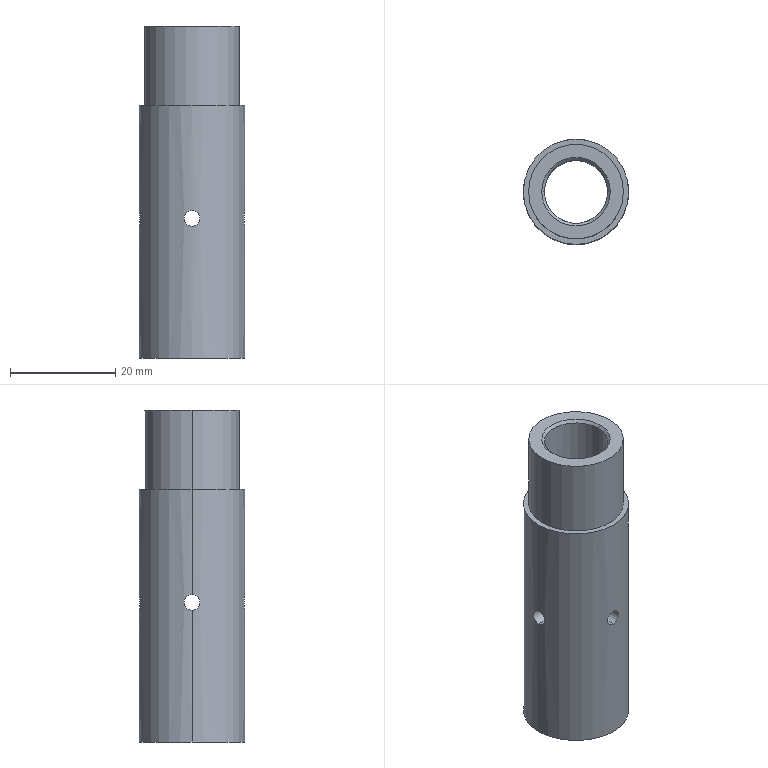Part | SolidWorks | features ICE 2, Chamfer 1, CirPattern 1, Extrusion 1, RevCut 1 | 1 solid | 19 faces | box 20 x 20 x 63 mm | volume 11653 mm3 | cylinder 14 | plane 3 | cone 2 | commonest cylinder face diameters 3 x8 12 x2 18 x2 20 x2
STEP:
#1=CARTESIAN_POINT('',(-6.,0.,62.5));
#2=VERTEX_POINT('',#1);
#3=CARTESIAN_POINT('',(6.,0.,62.5));
#4=VERTEX_POINT('',#3);
#5=CARTESIAN_POINT('',(0.,0.,62.5));
#6=DIRECTION('',(0.,0.,1.));
#7=DIRECTION('',(1.,0.,0.));
#8=AXIS2_PLACEMENT_3D('',#5,#6,#7);
#9=CIRCLE('',#8,6.);
#10=EDGE_CURVE('',#2,#4,#9,.T.);
#11=ORIENTED_EDGE('',*,*,#10,.F.);
#12=CARTESIAN_POINT('',(-6.5,0.,63.));
#13=VERTEX_POINT('',#12);
#14=CARTESIAN_POINT('',(-6.5,0.,63.));
#15=DIRECTION('',(-0.7071,0.,0.7071));
#16=VECTOR('',#15,1000.);
#17=LINE('',#14,#16);
#18=EDGE_CURVE('',#2,#13,#17,.T.);
#19=ORIENTED_EDGE('',*,*,#18,.T.);
#20=CARTESIAN_POINT('',(6.5,0.,63.));
#21=VERTEX_POINT('',#20);
#22=CARTESIAN_POINT('',(0.,0.,63.));
#23=DIRECTION('',(0.,0.,-1.));
#24=DIRECTION('',(1.,0.,0.));
#25=AXIS2_PLACEMENT_3D('',#22,#23,#24);
#26=CIRCLE('',#25,6.5);
#27=EDGE_CURVE('',#21,#13,#26,.T.);
#28=ORIENTED_EDGE('',*,*,#27,.F.);
#29=CARTESIAN_POINT('',(6.5,0.,63.));
#30=DIRECTION('',(0.7071,0.,0.7071));
#31=VECTOR('',#30,1000.);
#32=LINE('',#29,#31);
#33=EDGE_CURVE('',#4,#21,#32,.T.);
#34=ORIENTED_EDGE('',*,*,#33,.F.);
#35=EDGE_LOOP('',(#11,#19,#28,#34));
#36=FACE_OUTER_BOUND('',#35,.T.);
#37=CARTESIAN_POINT('',(0.,0.,63.));
#38=DIRECTION('',(0.,0.,1.));
#39=DIRECTION('',(1.,0.,0.));
#40=AXIS2_PLACEMENT_3D('',#37,#38,#39);
#41=CONICAL_SURFACE('',#40,6.5,0.7854);
#42=ADVANCED_FACE('',(#36),#41,.F.);
#43=CARTESIAN_POINT('',(-10.,0.,25.));
#44=VERTEX_POINT('',#43);
#45=CARTESIAN_POINT('',(-10.,0.,28.));
#46=VERTEX_POINT('',#45);
#47=CARTESIAN_POINT('',(-10.,0.,25.));
#48=CARTESIAN_POINT('',(-10.,0.1959,25.));
#49=CARTESIAN_POINT('',(-9.994,0.3935,25.039));
#50=CARTESIAN_POINT('',(-9.973,0.7546,25.189));
#51=CARTESIAN_POINT('',(-9.958,0.9216,25.3));
#52=CARTESIAN_POINT('',(-9.936,1.129,25.508));
#53=CARTESIAN_POINT('',(-9.929,1.192,25.585));
#54=CARTESIAN_POINT('',(-9.915,1.301,25.747));
#55=CARTESIAN_POINT('',(-9.909,1.347,25.834));
#56=CARTESIAN_POINT('',(-9.893,1.461,26.106));
#57=CARTESIAN_POINT('',(-9.887,1.5,26.301));
#58=CARTESIAN_POINT('',(-9.887,1.5,26.598));
#59=CARTESIAN_POINT('',(-9.888,1.49,26.696));
#60=CARTESIAN_POINT('',(-9.894,1.452,26.888));
#61=CARTESIAN_POINT('',(-9.898,1.423,26.983));
#62=CARTESIAN_POINT('',(-9.909,1.348,27.165));
#63=CARTESIAN_POINT('',(-9.915,1.302,27.251));
#64=CARTESIAN_POINT('',(-9.929,1.194,27.414));
#65=CARTESIAN_POINT('',(-9.936,1.13,27.491));
#66=CARTESIAN_POINT('',(-9.958,0.9234,27.698));
#67=CARTESIAN_POINT('',(-9.973,0.7563,27.81));
#68=CARTESIAN_POINT('',(-9.994,0.3956,27.96));
#69=CARTESIAN_POINT('',(-10.,0.1985,28.));
#70=CARTESIAN_POINT('',(-10.,0.,28.));
#71=B_SPLINE_CURVE_WITH_KNOTS('',3,(#47,#48,#49,#50,#51,#52,#53,#54,#55,#56,#57,#58,#59,#60,#61,#62,#63,#64,#65,#66,#67,#68,#69,#70),.UNSPECIFIED.,.F.,.F.,(4,2,2,2,2,2,2,2,2,2,2,4),(0.004696,0.005283,0.00587,0.006164,0.006457,0.007044,0.007337,0.007631,0.007924,0.008218,0.008805,0.009391),.UNSPECIFIED.);
#72=EDGE_CURVE('',#44,#46,#71,.T.);
#73=ORIENTED_EDGE('',*,*,#72,.F.);
#74=CARTESIAN_POINT('',(-6.,0.,25.));
#75=VERTEX_POINT('',#74);
#76=CARTESIAN_POINT('',(14.425,0.,25.));
#77=DIRECTION('',(1.,0.,0.));
#78=VECTOR('',#77,1000.);
#79=LINE('',#76,#78);
#80=EDGE_CURVE('',#44,#75,#79,.T.);
#81=ORIENTED_EDGE('',*,*,#80,.T.);
#82=CARTESIAN_POINT('',(-6.,0.,28.));
#83=VERTEX_POINT('',#82);
#84=CARTESIAN_POINT('',(-6.,0.,25.));
#85=CARTESIAN_POINT('',(-6.,0.1962,25.));
#86=CARTESIAN_POINT('',(-5.99,0.3943,25.04));
#87=CARTESIAN_POINT('',(-5.964,0.6653,25.152));
#88=CARTESIAN_POINT('',(-5.953,0.753,25.199));
#89=CARTESIAN_POINT('',(-5.93,0.9158,25.308));
#90=CARTESIAN_POINT('',(-5.918,0.9911,25.37));
#91=CARTESIAN_POINT('',(-5.893,1.129,25.508));
#92=CARTESIAN_POINT('',(-5.881,1.192,25.585));
#93=CARTESIAN_POINT('',(-5.858,1.301,25.747));
#94=CARTESIAN_POINT('',(-5.847,1.347,25.833));
#95=CARTESIAN_POINT('',(-5.82,1.461,26.106));
#96=CARTESIAN_POINT('',(-5.809,1.5,26.302));
#97=CARTESIAN_POINT('',(-5.809,1.5,26.598));
#98=CARTESIAN_POINT('',(-5.812,1.49,26.696));
#99=CARTESIAN_POINT('',(-5.822,1.452,26.889));
#100=CARTESIAN_POINT('',(-5.829,1.423,26.984));
#101=CARTESIAN_POINT('',(-5.856,1.31,27.256));
#102=CARTESIAN_POINT('',(-5.881,1.199,27.422));
#103=CARTESIAN_POINT('',(-5.93,0.9237,27.698));
#104=CARTESIAN_POINT('',(-5.955,0.7572,27.81));
#105=CARTESIAN_POINT('',(-5.981,0.4864,27.922));
#106=CARTESIAN_POINT('',(-5.988,0.3909,27.952));
#107=CARTESIAN_POINT('',(-5.998,0.1976,27.99));
#108=CARTESIAN_POINT('',(-6.,0.09951,28.));
#109=CARTESIAN_POINT('',(-6.,0.,28.));
#110=B_SPLINE_CURVE_WITH_KNOTS('',3,(#84,#85,#86,#87,#88,#89,#90,#91,#92,#93,#94,#95,#96,#97,#98,#99,#100,#101,#102,#103,#104,#105,#106,#107,#108,#109),.UNSPECIFIED.,.F.,.F.,(4,2,2,2,2,2,2,2,2,2,2,2,4),(0.004708,0.005297,0.005591,0.005885,0.006179,0.006474,0.007062,0.007356,0.00765,0.008239,0.008827,0.009121,0.009416),.UNSPECIFIED.);
#111=EDGE_CURVE('',#75,#83,#110,.T.);
#112=ORIENTED_EDGE('',*,*,#111,.T.);
#113=CARTESIAN_POINT('',(14.425,0.,28.));
#114=DIRECTION('',(1.,0.,0.));
#115=VECTOR('',#114,1000.);
#116=LINE('',#113,#115);
#117=EDGE_CURVE('',#46,#83,#116,.T.);
#118=ORIENTED_EDGE('',*,*,#117,.F.);
#119=EDGE_LOOP('',(#73,#81,#112,#118));
#120=FACE_OUTER_BOUND('',#119,.T.);
#121=CARTESIAN_POINT('',(14.425,0.,26.5));
#122=DIRECTION('',(1.,0.,0.));
#123=DIRECTION('',(0.,0.,1.));
#124=AXIS2_PLACEMENT_3D('',#121,#122,#123);
#125=CYLINDRICAL_SURFACE('',#124,1.5);
#126=ADVANCED_FACE('',(#120),#125,.F.);
#127=CARTESIAN_POINT('',(6.,0.,28.));
#128=VERTEX_POINT('',#127);
#129=CARTESIAN_POINT('',(6.,0.,25.));
#130=VERTEX_POINT('',#129);
#131=CARTESIAN_POINT('',(6.,0.,28.));
#132=CARTESIAN_POINT('',(6.,0.09953,28.));
#133=CARTESIAN_POINT('',(5.998,0.1973,27.99));
#134=CARTESIAN_POINT('',(5.988,0.3896,27.952));
#135=CARTESIAN_POINT('',(5.981,0.4851,27.923));
#136=CARTESIAN_POINT('',(5.964,0.6666,27.847));
#137=CARTESIAN_POINT('',(5.953,0.7526,27.801));
#138=CARTESIAN_POINT('',(5.93,0.9154,27.692));
#139=CARTESIAN_POINT('',(5.918,0.9921,27.629));
#140=CARTESIAN_POINT('',(5.881,1.199,27.423));
#141=CARTESIAN_POINT('',(5.856,1.31,27.256));
#142=CARTESIAN_POINT('',(5.82,1.46,26.895));
#143=CARTESIAN_POINT('',(5.809,1.5,26.697));
#144=CARTESIAN_POINT('',(5.809,1.5,26.402));
#145=CARTESIAN_POINT('',(5.812,1.49,26.302));
#146=CARTESIAN_POINT('',(5.822,1.452,26.11));
#147=CARTESIAN_POINT('',(5.829,1.423,26.016));
#148=CARTESIAN_POINT('',(5.856,1.31,25.743));
#149=CARTESIAN_POINT('',(5.881,1.199,25.578));
#150=CARTESIAN_POINT('',(5.918,0.9909,25.37));
#151=CARTESIAN_POINT('',(5.93,0.9156,25.308));
#152=CARTESIAN_POINT('',(5.953,0.7534,25.199));
#153=CARTESIAN_POINT('',(5.964,0.6656,25.152));
#154=CARTESIAN_POINT('',(5.981,0.4845,25.077));
#155=CARTESIAN_POINT('',(5.988,0.3909,25.048));
#156=CARTESIAN_POINT('',(5.998,0.1977,25.01));
#157=CARTESIAN_POINT('',(6.,0.09813,25.));
#158=CARTESIAN_POINT('',(6.,0.,25.));
#159=B_SPLINE_CURVE_WITH_KNOTS('',3,(#131,#132,#133,#134,#135,#136,#137,#138,#139,#140,#141,#142,#143,#144,#145,#146,#147,#148,#149,#150,#151,#152,#153,#154,#155,#156,#157,#158),.UNSPECIFIED.,.F.,.F.,(4,2,2,2,2,2,2,2,2,2,2,2,2,4),(0.,0.0002943,0.0005886,0.0008828,0.001177,0.001766,0.002354,0.002648,0.002943,0.003531,0.003826,0.00412,0.004414,0.004708),.UNSPECIFIED.);
#160=EDGE_CURVE('',#128,#130,#159,.T.);
#161=ORIENTED_EDGE('',*,*,#160,.T.);
#162=CARTESIAN_POINT('',(10.,0.,25.));
#163=VERTEX_POINT('',#162);
#164=CARTESIAN_POINT('',(14.425,0.,25.));
#165=DIRECTION('',(1.,0.,0.));
#166=VECTOR('',#165,1000.);
#167=LINE('',#164,#166);
#168=EDGE_CURVE('',#130,#163,#167,.T.);
#169=ORIENTED_EDGE('',*,*,#168,.T.);
#170=CARTESIAN_POINT('',(10.,0.,28.));
#171=VERTEX_POINT('',#170);
#172=CARTESIAN_POINT('',(10.,0.,28.));
#173=CARTESIAN_POINT('',(10.,0.09926,28.));
#174=CARTESIAN_POINT('',(9.999,0.1968,27.99));
#175=CARTESIAN_POINT('',(9.993,0.3888,27.952));
#176=CARTESIAN_POINT('',(9.989,0.4841,27.923));
#177=CARTESIAN_POINT('',(9.978,0.6657,27.848));
#178=CARTESIAN_POINT('',(9.972,0.7518,27.802));
#179=CARTESIAN_POINT('',(9.958,0.9148,27.693));
#180=CARTESIAN_POINT('',(9.951,0.9918,27.63));
#181=CARTESIAN_POINT('',(9.929,1.199,27.422));
#182=CARTESIAN_POINT('',(9.914,1.311,27.255));
#183=CARTESIAN_POINT('',(9.893,1.46,26.894));
#184=CARTESIAN_POINT('',(9.887,1.5,26.697));
#185=CARTESIAN_POINT('',(9.887,1.5,26.403));
#186=CARTESIAN_POINT('',(9.888,1.49,26.303));
#187=CARTESIAN_POINT('',(9.894,1.452,26.111));
#188=CARTESIAN_POINT('',(9.898,1.423,26.017));
#189=CARTESIAN_POINT('',(9.914,1.311,25.744));
#190=CARTESIAN_POINT('',(9.929,1.2,25.579));
#191=CARTESIAN_POINT('',(9.951,0.9908,25.369));
#192=CARTESIAN_POINT('',(9.958,0.9152,25.308));
#193=CARTESIAN_POINT('',(9.972,0.7529,25.199));
#194=CARTESIAN_POINT('',(9.978,0.6651,25.152));
#195=CARTESIAN_POINT('',(9.989,0.4835,25.077));
#196=CARTESIAN_POINT('',(9.993,0.39,25.048));
#197=CARTESIAN_POINT('',(9.999,0.1975,25.01));
#198=CARTESIAN_POINT('',(10.,0.09797,25.));
#199=CARTESIAN_POINT('',(10.,0.,25.));
#200=B_SPLINE_CURVE_WITH_KNOTS('',3,(#172,#173,#174,#175,#176,#177,#178,#179,#180,#181,#182,#183,#184,#185,#186,#187,#188,#189,#190,#191,#192,#193,#194,#195,#196,#197,#198,#199),.UNSPECIFIED.,.F.,.F.,(4,2,2,2,2,2,2,2,2,2,2,2,2,4),(0.,0.0002935,0.000587,0.0008806,0.001174,0.001761,0.002348,0.002642,0.002935,0.003522,0.003816,0.004109,0.004403,0.004696),.UNSPECIFIED.);
#201=EDGE_CURVE('',#171,#163,#200,.T.);
#202=ORIENTED_EDGE('',*,*,#201,.F.);
#203=CARTESIAN_POINT('',(14.425,0.,28.));
#204=DIRECTION('',(1.,0.,0.));
#205=VECTOR('',#204,1000.);
#206=LINE('',#203,#205);
#207=EDGE_CURVE('',#128,#171,#206,.T.);
#208=ORIENTED_EDGE('',*,*,#207,.F.);
#209=EDGE_LOOP('',(#161,#169,#202,#208));
#210=FACE_OUTER_BOUND('',#209,.T.);
#211=CARTESIAN_POINT('',(14.425,0.,26.5));
#212=DIRECTION('',(1.,0.,0.));
#213=DIRECTION('',(0.,0.,1.));
#214=AXIS2_PLACEMENT_3D('',#211,#212,#213);
#215=CYLINDRICAL_SURFACE('',#214,1.5);
#216=ADVANCED_FACE('',(#210),#215,.F.);
#217=CARTESIAN_POINT('',(0.,-10.,25.));
#218=VERTEX_POINT('',#217);
#219=CARTESIAN_POINT('',(0.,-10.,28.));
#220=VERTEX_POINT('',#219);
#221=CARTESIAN_POINT('',(0.,-10.,25.));
#222=CARTESIAN_POINT('',(-0.1959,-10.,25.));
#223=CARTESIAN_POINT('',(-0.3935,-9.994,25.039));
#224=CARTESIAN_POINT('',(-0.7546,-9.973,25.189));
#225=CARTESIAN_POINT('',(-0.9216,-9.958,25.3));
#226=CARTESIAN_POINT('',(-1.129,-9.936,25.508));
#227=CARTESIAN_POINT('',(-1.192,-9.929,25.585));
#228=CARTESIAN_POINT('',(-1.301,-9.915,25.747));
#229=CARTESIAN_POINT('',(-1.347,-9.909,25.834));
#230=CARTESIAN_POINT('',(-1.461,-9.893,26.106));
#231=CARTESIAN_POINT('',(-1.5,-9.887,26.301));
#232=CARTESIAN_POINT('',(-1.5,-9.887,26.598));
#233=CARTESIAN_POINT('',(-1.49,-9.888,26.696));
#234=CARTESIAN_POINT('',(-1.452,-9.894,26.888));
#235=CARTESIAN_POINT('',(-1.423,-9.898,26.983));
#236=CARTESIAN_POINT('',(-1.348,-9.909,27.165));
#237=CARTESIAN_POINT('',(-1.302,-9.915,27.251));
#238=CARTESIAN_POINT('',(-1.194,-9.929,27.414));
#239=CARTESIAN_POINT('',(-1.13,-9.936,27.491));
#240=CARTESIAN_POINT('',(-0.9234,-9.958,27.698));
#241=CARTESIAN_POINT('',(-0.7563,-9.973,27.81));
#242=CARTESIAN_POINT('',(-0.3956,-9.994,27.96));
#243=CARTESIAN_POINT('',(-0.1985,-10.,28.));
#244=CARTESIAN_POINT('',(0.,-10.,28.));
#245=B_SPLINE_CURVE_WITH_KNOTS('',3,(#221,#222,#223,#224,#225,#226,#227,#228,#229,#230,#231,#232,#233,#234,#235,#236,#237,#238,#239,#240,#241,#242,#243,#244),.UNSPECIFIED.,.F.,.F.,(4,2,2,2,2,2,2,2,2,2,2,4),(0.004696,0.005283,0.00587,0.006164,0.006457,0.007044,0.007337,0.007631,0.007924,0.008218,0.008805,0.009391),.UNSPECIFIED.);
#246=EDGE_CURVE('',#218,#220,#245,.T.);
#247=ORIENTED_EDGE('',*,*,#246,.F.);
#248=CARTESIAN_POINT('',(0.,-6.,25.));
#249=VERTEX_POINT('',#248);
#250=CARTESIAN_POINT('',(0.,14.425,25.));
#251=DIRECTION('',(0.,1.,0.));
#252=VECTOR('',#251,1000.);
#253=LINE('',#250,#252);
#254=EDGE_CURVE('',#218,#249,#253,.T.);
#255=ORIENTED_EDGE('',*,*,#254,.T.);
#256=CARTESIAN_POINT('',(0.,-6.,28.));
#257=VERTEX_POINT('',#256);
#258=CARTESIAN_POINT('',(0.,-6.,25.));
#259=CARTESIAN_POINT('',(-0.1962,-6.,25.));
#260=CARTESIAN_POINT('',(-0.3943,-5.99,25.04));
#261=CARTESIAN_POINT('',(-0.6653,-5.964,25.152));
#262=CARTESIAN_POINT('',(-0.753,-5.953,25.199));
#263=CARTESIAN_POINT('',(-0.9158,-5.93,25.308));
#264=CARTESIAN_POINT('',(-0.9911,-5.918,25.37));
#265=CARTESIAN_POINT('',(-1.129,-5.893,25.508));
#266=CARTESIAN_POINT('',(-1.192,-5.881,25.585));
#267=CARTESIAN_POINT('',(-1.301,-5.858,25.747));
#268=CARTESIAN_POINT('',(-1.347,-5.847,25.833));
#269=CARTESIAN_POINT('',(-1.461,-5.82,26.106));
#270=CARTESIAN_POINT('',(-1.5,-5.809,26.302));
#271=CARTESIAN_POINT('',(-1.5,-5.809,26.598));
#272=CARTESIAN_POINT('',(-1.49,-5.812,26.696));
#273=CARTESIAN_POINT('',(-1.452,-5.822,26.889));
#274=CARTESIAN_POINT('',(-1.423,-5.829,26.984));
#275=CARTESIAN_POINT('',(-1.31,-5.856,27.256));
#276=CARTESIAN_POINT('',(-1.199,-5.881,27.422));
#277=CARTESIAN_POINT('',(-0.9237,-5.93,27.698));
#278=CARTESIAN_POINT('',(-0.7572,-5.955,27.81));
#279=CARTESIAN_POINT('',(-0.4864,-5.981,27.922));
#280=CARTESIAN_POINT('',(-0.3909,-5.988,27.952));
#281=CARTESIAN_POINT('',(-0.1976,-5.998,27.99));
#282=CARTESIAN_POINT('',(-0.09951,-6.,28.));
#283=CARTESIAN_POINT('',(0.,-6.,28.));
#284=B_SPLINE_CURVE_WITH_KNOTS('',3,(#258,#259,#260,#261,#262,#263,#264,#265,#266,#267,#268,#269,#270,#271,#272,#273,#274,#275,#276,#277,#278,#279,#280,#281,#282,#283),.UNSPECIFIED.,.F.,.F.,(4,2,2,2,2,2,2,2,2,2,2,2,4),(0.004708,0.005297,0.005591,0.005885,0.006179,0.006474,0.007062,0.007356,0.00765,0.008239,0.008827,0.009121,0.009416),.UNSPECIFIED.);
#285=EDGE_CURVE('',#249,#257,#284,.T.);
#286=ORIENTED_EDGE('',*,*,#285,.T.);
#287=CARTESIAN_POINT('',(0.,14.425,28.));
#288=DIRECTION('',(0.,1.,0.));
#289=VECTOR('',#288,1000.);
#290=LINE('',#287,#289);
#291=EDGE_CURVE('',#220,#257,#290,.T.);
#292=ORIENTED_EDGE('',*,*,#291,.F.);
#293=EDGE_LOOP('',(#247,#255,#286,#292));
#294=FACE_OUTER_BOUND('',#293,.T.);
#295=CARTESIAN_POINT('',(0.,14.425,26.5));
#296=DIRECTION('',(0.,1.,0.));
#297=DIRECTION('',(0.,0.,1.));
#298=AXIS2_PLACEMENT_3D('',#295,#296,#297);
#299=CYLINDRICAL_SURFACE('',#298,1.5);
#300=ADVANCED_FACE('',(#294),#299,.F.);
#301=CARTESIAN_POINT('',(0.,6.,28.));
#302=VERTEX_POINT('',#301);
#303=CARTESIAN_POINT('',(0.,6.,25.));
#304=VERTEX_POINT('',#303);
#305=CARTESIAN_POINT('',(0.,6.,28.));
#306=CARTESIAN_POINT('',(-0.09953,6.,28.));
#307=CARTESIAN_POINT('',(-0.1973,5.998,27.99));
#308=CARTESIAN_POINT('',(-0.3896,5.988,27.952));
#309=CARTESIAN_POINT('',(-0.4851,5.981,27.923));
#310=CARTESIAN_POINT('',(-0.6666,5.964,27.847));
#311=CARTESIAN_POINT('',(-0.7526,5.953,27.801));
#312=CARTESIAN_POINT('',(-0.9154,5.93,27.692));
#313=CARTESIAN_POINT('',(-0.9921,5.918,27.629));
#314=CARTESIAN_POINT('',(-1.199,5.881,27.423));
#315=CARTESIAN_POINT('',(-1.31,5.856,27.256));
#316=CARTESIAN_POINT('',(-1.46,5.82,26.895));
#317=CARTESIAN_POINT('',(-1.5,5.809,26.697));
#318=CARTESIAN_POINT('',(-1.5,5.809,26.402));
#319=CARTESIAN_POINT('',(-1.49,5.812,26.302));
#320=CARTESIAN_POINT('',(-1.452,5.822,26.11));
#321=CARTESIAN_POINT('',(-1.423,5.829,26.016));
#322=CARTESIAN_POINT('',(-1.31,5.856,25.743));
#323=CARTESIAN_POINT('',(-1.199,5.881,25.578));
#324=CARTESIAN_POINT('',(-0.9909,5.918,25.37));
#325=CARTESIAN_POINT('',(-0.9156,5.93,25.308));
#326=CARTESIAN_POINT('',(-0.7534,5.953,25.199));
#327=CARTESIAN_POINT('',(-0.6656,5.964,25.152));
#328=CARTESIAN_POINT('',(-0.4845,5.981,25.077));
#329=CARTESIAN_POINT('',(-0.3909,5.988,25.048));
#330=CARTESIAN_POINT('',(-0.1977,5.998,25.01));
#331=CARTESIAN_POINT('',(-0.09813,6.,25.));
#332=CARTESIAN_POINT('',(0.,6.,25.));
#333=B_SPLINE_CURVE_WITH_KNOTS('',3,(#305,#306,#307,#308,#309,#310,#311,#312,#313,#314,#315,#316,#317,#318,#319,#320,#321,#322,#323,#324,#325,#326,#327,#328,#329,#330,#331,#332),.UNSPECIFIED.,.F.,.F.,(4,2,2,2,2,2,2,2,2,2,2,2,2,4),(0.,0.0002943,0.0005886,0.0008828,0.001177,0.001766,0.002354,0.002648,0.002943,0.003531,0.003826,0.00412,0.004414,0.004708),.UNSPECIFIED.);
#334=EDGE_CURVE('',#302,#304,#333,.T.);
#335=ORIENTED_EDGE('',*,*,#334,.T.);
#336=CARTESIAN_POINT('',(0.,10.,25.));
#337=VERTEX_POINT('',#336);
#338=CARTESIAN_POINT('',(0.,14.425,25.));
#339=DIRECTION('',(0.,1.,0.));
#340=VECTOR('',#339,1000.);
#341=LINE('',#338,#340);
#342=EDGE_CURVE('',#304,#337,#341,.T.);
#343=ORIENTED_EDGE('',*,*,#342,.T.);
#344=CARTESIAN_POINT('',(0.,10.,28.));
#345=VERTEX_POINT('',#344);
#346=CARTESIAN_POINT('',(0.,10.,28.));
#347=CARTESIAN_POINT('',(-0.09926,10.,28.));
#348=CARTESIAN_POINT('',(-0.1968,9.999,27.99));
#349=CARTESIAN_POINT('',(-0.3888,9.993,27.952));
#350=CARTESIAN_POINT('',(-0.4841,9.989,27.923));
#351=CARTESIAN_POINT('',(-0.6657,9.978,27.848));
#352=CARTESIAN_POINT('',(-0.7518,9.972,27.802));
#353=CARTESIAN_POINT('',(-0.9148,9.958,27.693));
#354=CARTESIAN_POINT('',(-0.9918,9.951,27.63));
#355=CARTESIAN_POINT('',(-1.199,9.929,27.422));
#356=CARTESIAN_POINT('',(-1.311,9.914,27.255));
#357=CARTESIAN_POINT('',(-1.46,9.893,26.894));
#358=CARTESIAN_POINT('',(-1.5,9.887,26.697));
#359=CARTESIAN_POINT('',(-1.5,9.887,26.403));
#360=CARTESIAN_POINT('',(-1.49,9.888,26.303));
#361=CARTESIAN_POINT('',(-1.452,9.894,26.111));
#362=CARTESIAN_POINT('',(-1.423,9.898,26.017));
#363=CARTESIAN_POINT('',(-1.311,9.914,25.744));
#364=CARTESIAN_POINT('',(-1.2,9.929,25.579));
#365=CARTESIAN_POINT('',(-0.9908,9.951,25.369));
#366=CARTESIAN_POINT('',(-0.9152,9.958,25.308));
#367=CARTESIAN_POINT('',(-0.7529,9.972,25.199));
#368=CARTESIAN_POINT('',(-0.6651,9.978,25.152));
#369=CARTESIAN_POINT('',(-0.4835,9.989,25.077));
#370=CARTESIAN_POINT('',(-0.39,9.993,25.048));
#371=CARTESIAN_POINT('',(-0.1975,9.999,25.01));
#372=CARTESIAN_POINT('',(-0.09797,10.,25.));
#373=CARTESIAN_POINT('',(0.,10.,25.));
#374=B_SPLINE_CURVE_WITH_KNOTS('',3,(#346,#347,#348,#349,#350,#351,#352,#353,#354,#355,#356,#357,#358,#359,#360,#361,#362,#363,#364,#365,#366,#367,#368,#369,#370,#371,#372,#373),.UNSPECIFIED.,.F.,.F.,(4,2,2,2,2,2,2,2,2,2,2,2,2,4),(0.,0.0002935,0.000587,0.0008806,0.001174,0.001761,0.002348,0.002642,0.002935,0.003522,0.003816,0.004109,0.004403,0.004696),.UNSPECIFIED.);
#375=EDGE_CURVE('',#345,#337,#374,.T.);
#376=ORIENTED_EDGE('',*,*,#375,.F.);
#377=CARTESIAN_POINT('',(0.,14.425,28.));
#378=DIRECTION('',(0.,1.,0.));
#379=VECTOR('',#378,1000.);
#380=LINE('',#377,#379);
#381=EDGE_CURVE('',#302,#345,#380,.T.);
#382=ORIENTED_EDGE('',*,*,#381,.F.);
#383=EDGE_LOOP('',(#335,#343,#376,#382));
#384=FACE_OUTER_BOUND('',#383,.T.);
#385=CARTESIAN_POINT('',(0.,14.425,26.5));
#386=DIRECTION('',(0.,1.,0.));
#387=DIRECTION('',(0.,0.,1.));
#388=AXIS2_PLACEMENT_3D('',#385,#386,#387);
#389=CYLINDRICAL_SURFACE('',#388,1.5);
#390=ADVANCED_FACE('',(#384),#389,.F.);
#391=CARTESIAN_POINT('',(9.,0.,63.));
#392=VERTEX_POINT('',#391);
#393=CARTESIAN_POINT('',(-9.,0.,63.));
#394=VERTEX_POINT('',#393);
#395=CARTESIAN_POINT('',(0.,0.,63.));
#396=DIRECTION('',(0.,0.,1.));
#397=DIRECTION('',(1.,0.,0.));
#398=AXIS2_PLACEMENT_3D('',#395,#396,#397);
#399=CIRCLE('',#398,9.);
#400=EDGE_CURVE('',#392,#394,#399,.T.);
#401=ORIENTED_EDGE('',*,*,#400,.F.);
#402=CARTESIAN_POINT('',(9.,0.,48.));
#403=VERTEX_POINT('',#402);
#404=CARTESIAN_POINT('',(9.,0.,63.));
#405=DIRECTION('',(0.,0.,-1.));
#406=VECTOR('',#405,1000.);
#407=LINE('',#404,#406);
#408=EDGE_CURVE('',#392,#403,#407,.T.);
#409=ORIENTED_EDGE('',*,*,#408,.T.);
#410=CARTESIAN_POINT('',(-9.,0.,48.));
#411=VERTEX_POINT('',#410);
#412=CARTESIAN_POINT('',(0.,0.,48.));
#413=DIRECTION('',(0.,0.,-1.));
#414=DIRECTION('',(-1.,0.,0.));
#415=AXIS2_PLACEMENT_3D('',#412,#413,#414);
#416=CIRCLE('',#415,9.);
#417=EDGE_CURVE('',#411,#403,#416,.T.);
#418=ORIENTED_EDGE('',*,*,#417,.F.);
#419=CARTESIAN_POINT('',(-9.,0.,63.));
#420=DIRECTION('',(0.,0.,-1.));
#421=VECTOR('',#420,1000.);
#422=LINE('',#419,#421);
#423=EDGE_CURVE('',#394,#411,#422,.T.);
#424=ORIENTED_EDGE('',*,*,#423,.F.);
#425=EDGE_LOOP('',(#401,#409,#418,#424));
#426=FACE_OUTER_BOUND('',#425,.T.);
#427=CARTESIAN_POINT('',(0.,0.,63.));
#428=DIRECTION('',(0.,0.,-1.));
#429=DIRECTION('',(-1.,0.,0.));
#430=AXIS2_PLACEMENT_3D('',#427,#428,#429);
#431=CYLINDRICAL_SURFACE('',#430,9.);
#432=ADVANCED_FACE('',(#426),#431,.T.);
#433=CARTESIAN_POINT('',(0.,-6.,28.));
#434=CARTESIAN_POINT('',(0.09953,-6.,28.));
#435=CARTESIAN_POINT('',(0.1973,-5.998,27.99));
#436=CARTESIAN_POINT('',(0.3896,-5.988,27.952));
#437=CARTESIAN_POINT('',(0.4851,-5.981,27.923));
#438=CARTESIAN_POINT('',(0.6666,-5.964,27.847));
#439=CARTESIAN_POINT('',(0.7526,-5.953,27.801));
#440=CARTESIAN_POINT('',(0.9154,-5.93,27.692));
#441=CARTESIAN_POINT('',(0.9921,-5.918,27.629));
#442=CARTESIAN_POINT('',(1.199,-5.881,27.423));
#443=CARTESIAN_POINT('',(1.31,-5.856,27.256));
#444=CARTESIAN_POINT('',(1.46,-5.82,26.895));
#445=CARTESIAN_POINT('',(1.5,-5.809,26.697));
#446=CARTESIAN_POINT('',(1.5,-5.809,26.402));
#447=CARTESIAN_POINT('',(1.49,-5.812,26.302));
#448=CARTESIAN_POINT('',(1.452,-5.822,26.11));
#449=CARTESIAN_POINT('',(1.423,-5.829,26.016));
#450=CARTESIAN_POINT('',(1.31,-5.856,25.743));
#451=CARTESIAN_POINT('',(1.199,-5.881,25.578));
#452=CARTESIAN_POINT('',(0.9909,-5.918,25.37));
#453=CARTESIAN_POINT('',(0.9156,-5.93,25.308));
#454=CARTESIAN_POINT('',(0.7534,-5.953,25.199));
#455=CARTESIAN_POINT('',(0.6656,-5.964,25.152));
#456=CARTESIAN_POINT('',(0.4845,-5.981,25.077));
#457=CARTESIAN_POINT('',(0.3909,-5.988,25.048));
#458=CARTESIAN_POINT('',(0.1977,-5.998,25.01));
#459=CARTESIAN_POINT('',(0.09813,-6.,25.));
#460=CARTESIAN_POINT('',(0.,-6.,25.));
#461=B_SPLINE_CURVE_WITH_KNOTS('',3,(#433,#434,#435,#436,#437,#438,#439,#440,#441,#442,#443,#444,#445,#446,#447,#448,#449,#450,#451,#452,#453,#454,#455,#456,#457,#458,#459,#460),.UNSPECIFIED.,.F.,.F.,(4,2,2,2,2,2,2,2,2,2,2,2,2,4),(0.,0.0002943,0.0005886,0.0008828,0.001177,0.001766,0.002354,0.002648,0.002943,0.003531,0.003826,0.00412,0.004414,0.004708),.UNSPECIFIED.);
#462=EDGE_CURVE('',#257,#249,#461,.T.);
#463=ORIENTED_EDGE('',*,*,#462,.F.);
#464=ORIENTED_EDGE('',*,*,#285,.F.);
#465=EDGE_LOOP('',(#463,#464));
#466=FACE_BOUND('',#465,.T.);
#467=ORIENTED_EDGE('',*,*,#10,.T.);
#468=CARTESIAN_POINT('',(6.,0.,63.));
#469=DIRECTION('',(0.,0.,-1.));
#470=VECTOR('',#469,1000.);
#471=LINE('',#468,#470);
#472=EDGE_CURVE('',#4,#128,#471,.T.);
#473=ORIENTED_EDGE('',*,*,#472,.T.);
#474=CARTESIAN_POINT('',(6.,0.,25.));
#475=CARTESIAN_POINT('',(6.,-0.1962,25.));
#476=CARTESIAN_POINT('',(5.99,-0.3943,25.04));
#477=CARTESIAN_POINT('',(5.964,-0.6653,25.152));
#478=CARTESIAN_POINT('',(5.953,-0.753,25.199));
#479=CARTESIAN_POINT('',(5.93,-0.9158,25.308));
#480=CARTESIAN_POINT('',(5.918,-0.9911,25.37));
#481=CARTESIAN_POINT('',(5.893,-1.129,25.508));
#482=CARTESIAN_POINT('',(5.881,-1.192,25.585));
#483=CARTESIAN_POINT('',(5.858,-1.301,25.747));
#484=CARTESIAN_POINT('',(5.847,-1.347,25.833));
#485=CARTESIAN_POINT('',(5.82,-1.461,26.106));
#486=CARTESIAN_POINT('',(5.809,-1.5,26.302));
#487=CARTESIAN_POINT('',(5.809,-1.5,26.598));
#488=CARTESIAN_POINT('',(5.812,-1.49,26.696));
#489=CARTESIAN_POINT('',(5.822,-1.452,26.889));
#490=CARTESIAN_POINT('',(5.829,-1.423,26.984));
#491=CARTESIAN_POINT('',(5.856,-1.31,27.256));
#492=CARTESIAN_POINT('',(5.881,-1.199,27.422));
#493=CARTESIAN_POINT('',(5.93,-0.9237,27.698));
#494=CARTESIAN_POINT('',(5.955,-0.7572,27.81));
#495=CARTESIAN_POINT('',(5.981,-0.4864,27.922));
#496=CARTESIAN_POINT('',(5.988,-0.3909,27.952));
#497=CARTESIAN_POINT('',(5.998,-0.1976,27.99));
#498=CARTESIAN_POINT('',(6.,-0.09951,28.));
#499=CARTESIAN_POINT('',(6.,0.,28.));
#500=B_SPLINE_CURVE_WITH_KNOTS('',3,(#474,#475,#476,#477,#478,#479,#480,#481,#482,#483,#484,#485,#486,#487,#488,#489,#490,#491,#492,#493,#494,#495,#496,#497,#498,#499),.UNSPECIFIED.,.F.,.F.,(4,2,2,2,2,2,2,2,2,2,2,2,4),(0.004708,0.005297,0.005591,0.005885,0.006179,0.006474,0.007062,0.007356,0.00765,0.008239,0.008827,0.009121,0.009416),.UNSPECIFIED.);
#501=EDGE_CURVE('',#130,#128,#500,.T.);
#502=ORIENTED_EDGE('',*,*,#501,.F.);
#503=CARTESIAN_POINT('',(6.,0.,0.));
#504=VERTEX_POINT('',#503);
#505=CARTESIAN_POINT('',(6.,0.,63.));
#506=DIRECTION('',(0.,0.,-1.));
#507=VECTOR('',#506,1000.);
#508=LINE('',#505,#507);
#509=EDGE_CURVE('',#130,#504,#508,.T.);
#510=ORIENTED_EDGE('',*,*,#509,.T.);
#511=CARTESIAN_POINT('',(-6.,0.,0.));
#512=VERTEX_POINT('',#511);
#513=CARTESIAN_POINT('',(0.,0.,0.));
#514=DIRECTION('',(0.,0.,-1.));
#515=DIRECTION('',(-1.,0.,0.));
#516=AXIS2_PLACEMENT_3D('',#513,#514,#515);
#517=CIRCLE('',#516,6.);
#518=EDGE_CURVE('',#504,#512,#517,.T.);
#519=ORIENTED_EDGE('',*,*,#518,.T.);
#520=CARTESIAN_POINT('',(-6.,0.,63.));
#521=DIRECTION('',(0.,0.,-1.));
#522=VECTOR('',#521,1000.);
#523=LINE('',#520,#522);
#524=EDGE_CURVE('',#75,#512,#523,.T.);
#525=ORIENTED_EDGE('',*,*,#524,.F.);
#526=CARTESIAN_POINT('',(-6.,0.,28.));
#527=CARTESIAN_POINT('',(-6.,-0.09953,28.));
#528=CARTESIAN_POINT('',(-5.998,-0.1973,27.99));
#529=CARTESIAN_POINT('',(-5.988,-0.3896,27.952));
#530=CARTESIAN_POINT('',(-5.981,-0.4851,27.923));
#531=CARTESIAN_POINT('',(-5.964,-0.6666,27.847));
#532=CARTESIAN_POINT('',(-5.953,-0.7526,27.801));
#533=CARTESIAN_POINT('',(-5.93,-0.9154,27.692));
#534=CARTESIAN_POINT('',(-5.918,-0.9921,27.629));
#535=CARTESIAN_POINT('',(-5.881,-1.199,27.423));
#536=CARTESIAN_POINT('',(-5.856,-1.31,27.256));
#537=CARTESIAN_POINT('',(-5.82,-1.46,26.895));
#538=CARTESIAN_POINT('',(-5.809,-1.5,26.697));
#539=CARTESIAN_POINT('',(-5.809,-1.5,26.402));
#540=CARTESIAN_POINT('',(-5.812,-1.49,26.302));
#541=CARTESIAN_POINT('',(-5.822,-1.452,26.11));
#542=CARTESIAN_POINT('',(-5.829,-1.423,26.016));
#543=CARTESIAN_POINT('',(-5.856,-1.31,25.743));
#544=CARTESIAN_POINT('',(-5.881,-1.199,25.578));
#545=CARTESIAN_POINT('',(-5.918,-0.9909,25.37));
#546=CARTESIAN_POINT('',(-5.93,-0.9156,25.308));
#547=CARTESIAN_POINT('',(-5.953,-0.7534,25.199));
#548=CARTESIAN_POINT('',(-5.964,-0.6656,25.152));
#549=CARTESIAN_POINT('',(-5.981,-0.4845,25.077));
#550=CARTESIAN_POINT('',(-5.988,-0.3909,25.048));
#551=CARTESIAN_POINT('',(-5.998,-0.1977,25.01));
#552=CARTESIAN_POINT('',(-6.,-0.09813,25.));
#553=CARTESIAN_POINT('',(-6.,0.,25.));
#554=B_SPLINE_CURVE_WITH_KNOTS('',3,(#526,#527,#528,#529,#530,#531,#532,#533,#534,#535,#536,#537,#538,#539,#540,#541,#542,#543,#544,#545,#546,#547,#548,#549,#550,#551,#552,#553),.UNSPECIFIED.,.F.,.F.,(4,2,2,2,2,2,2,2,2,2,2,2,2,4),(0.,0.0002943,0.0005886,0.0008828,0.001177,0.001766,0.002354,0.002648,0.002943,0.003531,0.003826,0.00412,0.004414,0.004708),.UNSPECIFIED.);
#555=EDGE_CURVE('',#83,#75,#554,.T.);
#556=ORIENTED_EDGE('',*,*,#555,.F.);
#557=CARTESIAN_POINT('',(-6.,0.,63.));
#558=DIRECTION('',(0.,0.,-1.));
#559=VECTOR('',#558,1000.);
#560=LINE('',#557,#559);
#561=EDGE_CURVE('',#2,#83,#560,.T.);
#562=ORIENTED_EDGE('',*,*,#561,.F.);
#563=EDGE_LOOP('',(#467,#473,#502,#510,#519,#525,#556,#562));
#564=FACE_OUTER_BOUND('',#563,.T.);
#565=CARTESIAN_POINT('',(0.,0.,63.));
#566=DIRECTION('',(0.,0.,-1.));
#567=DIRECTION('',(-1.,0.,0.));
#568=AXIS2_PLACEMENT_3D('',#565,#566,#567);
#569=CYLINDRICAL_SURFACE('',#568,6.);
#570=ADVANCED_FACE('',(#466,#564),#569,.F.);
#571=ORIENTED_EDGE('',*,*,#375,.T.);
#572=CARTESIAN_POINT('',(0.,10.,25.));
#573=CARTESIAN_POINT('',(0.1959,10.,25.));
#574=CARTESIAN_POINT('',(0.3935,9.994,25.039));
#575=CARTESIAN_POINT('',(0.7546,9.973,25.189));
#576=CARTESIAN_POINT('',(0.9216,9.958,25.3));
#577=CARTESIAN_POINT('',(1.129,9.936,25.508));
#578=CARTESIAN_POINT('',(1.192,9.929,25.585));
#579=CARTESIAN_POINT('',(1.301,9.915,25.747));
#580=CARTESIAN_POINT('',(1.347,9.909,25.834));
#581=CARTESIAN_POINT('',(1.461,9.893,26.106));
#582=CARTESIAN_POINT('',(1.5,9.887,26.301));
#583=CARTESIAN_POINT('',(1.5,9.887,26.598));
#584=CARTESIAN_POINT('',(1.49,9.888,26.696));
#585=CARTESIAN_POINT('',(1.452,9.894,26.888));
#586=CARTESIAN_POINT('',(1.423,9.898,26.983));
#587=CARTESIAN_POINT('',(1.348,9.909,27.165));
#588=CARTESIAN_POINT('',(1.302,9.915,27.251));
#589=CARTESIAN_POINT('',(1.194,9.929,27.414));
#590=CARTESIAN_POINT('',(1.13,9.936,27.491));
#591=CARTESIAN_POINT('',(0.9234,9.958,27.698));
#592=CARTESIAN_POINT('',(0.7563,9.973,27.81));
#593=CARTESIAN_POINT('',(0.3956,9.994,27.96));
#594=CARTESIAN_POINT('',(0.1985,10.,28.));
#595=CARTESIAN_POINT('',(0.,10.,28.));
#596=B_SPLINE_CURVE_WITH_KNOTS('',3,(#572,#573,#574,#575,#576,#577,#578,#579,#580,#581,#582,#583,#584,#585,#586,#587,#588,#589,#590,#591,#592,#593,#594,#595),.UNSPECIFIED.,.F.,.F.,(4,2,2,2,2,2,2,2,2,2,2,4),(0.004696,0.005283,0.00587,0.006164,0.006457,0.007044,0.007337,0.007631,0.007924,0.008218,0.008805,0.009391),.UNSPECIFIED.);
#597=EDGE_CURVE('',#337,#345,#596,.T.);
#598=ORIENTED_EDGE('',*,*,#597,.T.);
#599=EDGE_LOOP('',(#571,#598));
#600=FACE_BOUND('',#599,.T.);
#601=CARTESIAN_POINT('',(-10.,0.,48.));
#602=VERTEX_POINT('',#601);
#603=CARTESIAN_POINT('',(10.,0.,48.));
#604=VERTEX_POINT('',#603);
#605=CARTESIAN_POINT('',(0.,0.,48.));
#606=DIRECTION('',(0.,0.,-1.));
#607=DIRECTION('',(-1.,0.,0.));
#608=AXIS2_PLACEMENT_3D('',#605,#606,#607);
#609=CIRCLE('',#608,10.);
#610=EDGE_CURVE('',#602,#604,#609,.T.);
#611=ORIENTED_EDGE('',*,*,#610,.T.);
#612=CARTESIAN_POINT('',(10.,0.,48.));
#613=DIRECTION('',(0.,0.,-1.));
#614=VECTOR('',#613,1000.);
#615=LINE('',#612,#614);
#616=EDGE_CURVE('',#604,#171,#615,.T.);
#617=ORIENTED_EDGE('',*,*,#616,.T.);
#618=ORIENTED_EDGE('',*,*,#201,.T.);
#619=CARTESIAN_POINT('',(10.,0.,0.));
#620=VERTEX_POINT('',#619);
#621=CARTESIAN_POINT('',(10.,0.,48.));
#622=DIRECTION('',(0.,0.,-1.));
#623=VECTOR('',#622,1000.);
#624=LINE('',#621,#623);
#625=EDGE_CURVE('',#163,#620,#624,.T.);
#626=ORIENTED_EDGE('',*,*,#625,.T.);
#627=CARTESIAN_POINT('',(-10.,0.,0.));
#628=VERTEX_POINT('',#627);
#629=CARTESIAN_POINT('',(0.,0.,0.));
#630=DIRECTION('',(0.,0.,-1.));
#631=DIRECTION('',(-1.,0.,0.));
#632=AXIS2_PLACEMENT_3D('',#629,#630,#631);
#633=CIRCLE('',#632,10.);
#634=EDGE_CURVE('',#628,#620,#633,.T.);
#635=ORIENTED_EDGE('',*,*,#634,.F.);
#636=CARTESIAN_POINT('',(-10.,0.,48.));
#637=DIRECTION('',(0.,0.,-1.));
#638=VECTOR('',#637,1000.);
#639=LINE('',#636,#638);
#640=EDGE_CURVE('',#44,#628,#639,.T.);
#641=ORIENTED_EDGE('',*,*,#640,.F.);
#642=ORIENTED_EDGE('',*,*,#72,.T.);
#643=CARTESIAN_POINT('',(-10.,0.,48.));
#644=DIRECTION('',(0.,0.,-1.));
#645=VECTOR('',#644,1000.);
#646=LINE('',#643,#645);
#647=EDGE_CURVE('',#602,#46,#646,.T.);
#648=ORIENTED_EDGE('',*,*,#647,.F.);
#649=EDGE_LOOP('',(#611,#617,#618,#626,#635,#641,#642,#648));
#650=FACE_OUTER_BOUND('',#649,.T.);
#651=CARTESIAN_POINT('',(0.,0.,48.));
#652=DIRECTION('',(0.,0.,-1.));
#653=DIRECTION('',(-1.,0.,0.));
#654=AXIS2_PLACEMENT_3D('',#651,#652,#653);
#655=CYLINDRICAL_SURFACE('',#654,10.);
#656=ADVANCED_FACE('',(#600,#650),#655,.T.);
#657=ORIENTED_EDGE('',*,*,#616,.F.);
#658=CARTESIAN_POINT('',(0.,0.,48.));
#659=DIRECTION('',(0.,0.,-1.));
#660=DIRECTION('',(-1.,0.,0.));
#661=AXIS2_PLACEMENT_3D('',#658,#659,#660);
#662=CIRCLE('',#661,10.);
#663=EDGE_CURVE('',#604,#602,#662,.T.);
#664=ORIENTED_EDGE('',*,*,#663,.T.);
#665=ORIENTED_EDGE('',*,*,#647,.T.);
#666=CARTESIAN_POINT('',(-10.,0.,28.));
#667=CARTESIAN_POINT('',(-10.,-0.09926,28.));
#668=CARTESIAN_POINT('',(-9.999,-0.1968,27.99));
#669=CARTESIAN_POINT('',(-9.993,-0.3888,27.952));
#670=CARTESIAN_POINT('',(-9.989,-0.4841,27.923));
#671=CARTESIAN_POINT('',(-9.978,-0.6657,27.848));
#672=CARTESIAN_POINT('',(-9.972,-0.7518,27.802));
#673=CARTESIAN_POINT('',(-9.958,-0.9148,27.693));
#674=CARTESIAN_POINT('',(-9.951,-0.9918,27.63));
#675=CARTESIAN_POINT('',(-9.929,-1.199,27.422));
#676=CARTESIAN_POINT('',(-9.914,-1.311,27.255));
#677=CARTESIAN_POINT('',(-9.893,-1.46,26.894));
#678=CARTESIAN_POINT('',(-9.887,-1.5,26.697));
#679=CARTESIAN_POINT('',(-9.887,-1.5,26.403));
#680=CARTESIAN_POINT('',(-9.888,-1.49,26.303));
#681=CARTESIAN_POINT('',(-9.894,-1.452,26.111));
#682=CARTESIAN_POINT('',(-9.898,-1.423,26.017));
#683=CARTESIAN_POINT('',(-9.914,-1.311,25.744));
#684=CARTESIAN_POINT('',(-9.929,-1.2,25.579));
#685=CARTESIAN_POINT('',(-9.951,-0.9908,25.369));
#686=CARTESIAN_POINT('',(-9.958,-0.9152,25.308));
#687=CARTESIAN_POINT('',(-9.972,-0.7529,25.199));
#688=CARTESIAN_POINT('',(-9.978,-0.6651,25.152));
#689=CARTESIAN_POINT('',(-9.989,-0.4835,25.077));
#690=CARTESIAN_POINT('',(-9.993,-0.39,25.048));
#691=CARTESIAN_POINT('',(-9.999,-0.1975,25.01));
#692=CARTESIAN_POINT('',(-10.,-0.09797,25.));
#693=CARTESIAN_POINT('',(-10.,0.,25.));
#694=B_SPLINE_CURVE_WITH_KNOTS('',3,(#666,#667,#668,#669,#670,#671,#672,#673,#674,#675,#676,#677,#678,#679,#680,#681,#682,#683,#684,#685,#686,#687,#688,#689,#690,#691,#692,#693),.UNSPECIFIED.,.F.,.F.,(4,2,2,2,2,2,2,2,2,2,2,2,2,4),(0.,0.0002935,0.000587,0.0008806,0.001174,0.001761,0.002348,0.002642,0.002935,0.003522,0.003816,0.004109,0.004403,0.004696),.UNSPECIFIED.);
#695=EDGE_CURVE('',#46,#44,#694,.T.);
#696=ORIENTED_EDGE('',*,*,#695,.T.);
#697=ORIENTED_EDGE('',*,*,#640,.T.);
#698=CARTESIAN_POINT('',(0.,0.,0.));
#699=DIRECTION('',(0.,0.,-1.));
#700=DIRECTION('',(-1.,0.,0.));
#701=AXIS2_PLACEMENT_3D('',#698,#699,#700);
#702=CIRCLE('',#701,10.);
#703=EDGE_CURVE('',#620,#628,#702,.T.);
#704=ORIENTED_EDGE('',*,*,#703,.F.);
#705=ORIENTED_EDGE('',*,*,#625,.F.);
#706=CARTESIAN_POINT('',(10.,0.,25.));
#707=CARTESIAN_POINT('',(10.,-0.1959,25.));
#708=CARTESIAN_POINT('',(9.994,-0.3935,25.039));
#709=CARTESIAN_POINT('',(9.973,-0.7546,25.189));
#710=CARTESIAN_POINT('',(9.958,-0.9216,25.3));
#711=CARTESIAN_POINT('',(9.936,-1.129,25.508));
#712=CARTESIAN_POINT('',(9.929,-1.192,25.585));
#713=CARTESIAN_POINT('',(9.915,-1.301,25.747));
#714=CARTESIAN_POINT('',(9.909,-1.347,25.834));
#715=CARTESIAN_POINT('',(9.893,-1.461,26.106));
#716=CARTESIAN_POINT('',(9.887,-1.5,26.301));
#717=CARTESIAN_POINT('',(9.887,-1.5,26.598));
#718=CARTESIAN_POINT('',(9.888,-1.49,26.696));
#719=CARTESIAN_POINT('',(9.894,-1.452,26.888));
#720=CARTESIAN_POINT('',(9.898,-1.423,26.983));
#721=CARTESIAN_POINT('',(9.909,-1.348,27.165));
#722=CARTESIAN_POINT('',(9.915,-1.302,27.251));
#723=CARTESIAN_POINT('',(9.929,-1.194,27.414));
#724=CARTESIAN_POINT('',(9.936,-1.13,27.491));
#725=CARTESIAN_POINT('',(9.958,-0.9234,27.698));
#726=CARTESIAN_POINT('',(9.973,-0.7563,27.81));
#727=CARTESIAN_POINT('',(9.994,-0.3956,27.96));
#728=CARTESIAN_POINT('',(10.,-0.1985,28.));
#729=CARTESIAN_POINT('',(10.,0.,28.));
#730=B_SPLINE_CURVE_WITH_KNOTS('',3,(#706,#707,#708,#709,#710,#711,#712,#713,#714,#715,#716,#717,#718,#719,#720,#721,#722,#723,#724,#725,#726,#727,#728,#729),.UNSPECIFIED.,.F.,.F.,(4,2,2,2,2,2,2,2,2,2,2,4),(0.004696,0.005283,0.00587,0.006164,0.006457,0.007044,0.007337,0.007631,0.007924,0.008218,0.008805,0.009391),.UNSPECIFIED.);
#731=EDGE_CURVE('',#163,#171,#730,.T.);
#732=ORIENTED_EDGE('',*,*,#731,.T.);
#733=EDGE_LOOP('',(#657,#664,#665,#696,#697,#704,#705,#732));
#734=FACE_OUTER_BOUND('',#733,.T.);
#735=CARTESIAN_POINT('',(0.,-10.,28.));
#736=CARTESIAN_POINT('',(0.09926,-10.,28.));
#737=CARTESIAN_POINT('',(0.1968,-9.999,27.99));
#738=CARTESIAN_POINT('',(0.3888,-9.993,27.952));
#739=CARTESIAN_POINT('',(0.4841,-9.989,27.923));
#740=CARTESIAN_POINT('',(0.6657,-9.978,27.848));
#741=CARTESIAN_POINT('',(0.7518,-9.972,27.802));
#742=CARTESIAN_POINT('',(0.9148,-9.958,27.693));
#743=CARTESIAN_POINT('',(0.9918,-9.951,27.63));
#744=CARTESIAN_POINT('',(1.199,-9.929,27.422));
#745=CARTESIAN_POINT('',(1.311,-9.914,27.255));
#746=CARTESIAN_POINT('',(1.46,-9.893,26.894));
#747=CARTESIAN_POINT('',(1.5,-9.887,26.697));
#748=CARTESIAN_POINT('',(1.5,-9.887,26.403));
#749=CARTESIAN_POINT('',(1.49,-9.888,26.303));
#750=CARTESIAN_POINT('',(1.452,-9.894,26.111));
#751=CARTESIAN_POINT('',(1.423,-9.898,26.017));
#752=CARTESIAN_POINT('',(1.311,-9.914,25.744));
#753=CARTESIAN_POINT('',(1.2,-9.929,25.579));
#754=CARTESIAN_POINT('',(0.9908,-9.951,25.369));
#755=CARTESIAN_POINT('',(0.9152,-9.958,25.308));
#756=CARTESIAN_POINT('',(0.7529,-9.972,25.199));
#757=CARTESIAN_POINT('',(0.6651,-9.978,25.152));
#758=CARTESIAN_POINT('',(0.4835,-9.989,25.077));
#759=CARTESIAN_POINT('',(0.39,-9.993,25.048));
#760=CARTESIAN_POINT('',(0.1975,-9.999,25.01));
#761=CARTESIAN_POINT('',(0.09797,-10.,25.));
#762=CARTESIAN_POINT('',(0.,-10.,25.));
#763=B_SPLINE_CURVE_WITH_KNOTS('',3,(#735,#736,#737,#738,#739,#740,#741,#742,#743,#744,#745,#746,#747,#748,#749,#750,#751,#752,#753,#754,#755,#756,#757,#758,#759,#760,#761,#762),.UNSPECIFIED.,.F.,.F.,(4,2,2,2,2,2,2,2,2,2,2,2,2,4),(0.,0.0002935,0.000587,0.0008806,0.001174,0.001761,0.002348,0.002642,0.002935,0.003522,0.003816,0.004109,0.004403,0.004696),.UNSPECIFIED.);
#764=EDGE_CURVE('',#220,#218,#763,.T.);
#765=ORIENTED_EDGE('',*,*,#764,.T.);
#766=ORIENTED_EDGE('',*,*,#246,.T.);
#767=EDGE_LOOP('',(#765,#766));
#768=FACE_BOUND('',#767,.T.);
#769=CARTESIAN_POINT('',(0.,0.,48.));
#770=DIRECTION('',(0.,0.,-1.));
#771=DIRECTION('',(-1.,0.,0.));
#772=AXIS2_PLACEMENT_3D('',#769,#770,#771);
#773=CYLINDRICAL_SURFACE('',#772,10.);
#774=ADVANCED_FACE('',(#734,#768),#773,.T.);
#775=ORIENTED_EDGE('',*,*,#472,.F.);
#776=CARTESIAN_POINT('',(0.,0.,62.5));
#777=DIRECTION('',(0.,0.,1.));
#778=DIRECTION('',(1.,0.,0.));
#779=AXIS2_PLACEMENT_3D('',#776,#777,#778);
#780=CIRCLE('',#779,6.);
#781=EDGE_CURVE('',#4,#2,#780,.T.);
#782=ORIENTED_EDGE('',*,*,#781,.T.);
#783=ORIENTED_EDGE('',*,*,#561,.T.);
#784=ORIENTED_EDGE('',*,*,#111,.F.);
#785=ORIENTED_EDGE('',*,*,#524,.T.);
#786=CARTESIAN_POINT('',(0.,0.,0.));
#787=DIRECTION('',(0.,0.,-1.));
#788=DIRECTION('',(-1.,0.,0.));
#789=AXIS2_PLACEMENT_3D('',#786,#787,#788);
#790=CIRCLE('',#789,6.);
#791=EDGE_CURVE('',#512,#504,#790,.T.);
#792=ORIENTED_EDGE('',*,*,#791,.T.);
#793=ORIENTED_EDGE('',*,*,#509,.F.);
#794=ORIENTED_EDGE('',*,*,#160,.F.);
#795=EDGE_LOOP('',(#775,#782,#783,#784,#785,#792,#793,#794));
#796=FACE_OUTER_BOUND('',#795,.T.);
#797=ORIENTED_EDGE('',*,*,#334,.F.);
#798=CARTESIAN_POINT('',(0.,6.,25.));
#799=CARTESIAN_POINT('',(0.1962,6.,25.));
#800=CARTESIAN_POINT('',(0.3943,5.99,25.04));
#801=CARTESIAN_POINT('',(0.6653,5.964,25.152));
#802=CARTESIAN_POINT('',(0.753,5.953,25.199));
#803=CARTESIAN_POINT('',(0.9158,5.93,25.308));
#804=CARTESIAN_POINT('',(0.9911,5.918,25.37));
#805=CARTESIAN_POINT('',(1.129,5.893,25.508));
#806=CARTESIAN_POINT('',(1.192,5.881,25.585));
#807=CARTESIAN_POINT('',(1.301,5.858,25.747));
#808=CARTESIAN_POINT('',(1.347,5.847,25.833));
#809=CARTESIAN_POINT('',(1.461,5.82,26.106));
#810=CARTESIAN_POINT('',(1.5,5.809,26.302));
#811=CARTESIAN_POINT('',(1.5,5.809,26.598));
#812=CARTESIAN_POINT('',(1.49,5.812,26.696));
#813=CARTESIAN_POINT('',(1.452,5.822,26.889));
#814=CARTESIAN_POINT('',(1.423,5.829,26.984));
#815=CARTESIAN_POINT('',(1.31,5.856,27.256));
#816=CARTESIAN_POINT('',(1.199,5.881,27.422));
#817=CARTESIAN_POINT('',(0.9237,5.93,27.698));
#818=CARTESIAN_POINT('',(0.7572,5.955,27.81));
#819=CARTESIAN_POINT('',(0.4864,5.981,27.922));
#820=CARTESIAN_POINT('',(0.3909,5.988,27.952));
#821=CARTESIAN_POINT('',(0.1976,5.998,27.99));
#822=CARTESIAN_POINT('',(0.09951,6.,28.));
#823=CARTESIAN_POINT('',(0.,6.,28.));
#824=B_SPLINE_CURVE_WITH_KNOTS('',3,(#798,#799,#800,#801,#802,#803,#804,#805,#806,#807,#808,#809,#810,#811,#812,#813,#814,#815,#816,#817,#818,#819,#820,#821,#822,#823),.UNSPECIFIED.,.F.,.F.,(4,2,2,2,2,2,2,2,2,2,2,2,4),(0.004708,0.005297,0.005591,0.005885,0.006179,0.006474,0.007062,0.007356,0.00765,0.008239,0.008827,0.009121,0.009416),.UNSPECIFIED.);
#825=EDGE_CURVE('',#304,#302,#824,.T.);
#826=ORIENTED_EDGE('',*,*,#825,.F.);
#827=EDGE_LOOP('',(#797,#826));
#828=FACE_BOUND('',#827,.T.);
#829=CARTESIAN_POINT('',(0.,0.,63.));
#830=DIRECTION('',(0.,0.,-1.));
#831=DIRECTION('',(-1.,0.,0.));
#832=AXIS2_PLACEMENT_3D('',#829,#830,#831);
#833=CYLINDRICAL_SURFACE('',#832,6.);
#834=ADVANCED_FACE('',(#796,#828),#833,.F.);
#835=ORIENTED_EDGE('',*,*,#408,.F.);
#836=CARTESIAN_POINT('',(0.,0.,63.));
#837=DIRECTION('',(0.,0.,1.));
#838=DIRECTION('',(1.,0.,0.));
#839=AXIS2_PLACEMENT_3D('',#836,#837,#838);
#840=CIRCLE('',#839,9.);
#841=EDGE_CURVE('',#394,#392,#840,.T.);
#842=ORIENTED_EDGE('',*,*,#841,.F.);
#843=ORIENTED_EDGE('',*,*,#423,.T.);
#844=CARTESIAN_POINT('',(0.,0.,48.));
#845=DIRECTION('',(0.,0.,-1.));
#846=DIRECTION('',(-1.,0.,0.));
#847=AXIS2_PLACEMENT_3D('',#844,#845,#846);
#848=CIRCLE('',#847,9.);
#849=EDGE_CURVE('',#403,#411,#848,.T.);
#850=ORIENTED_EDGE('',*,*,#849,.F.);
#851=EDGE_LOOP('',(#835,#842,#843,#850));
#852=FACE_OUTER_BOUND('',#851,.T.);
#853=CARTESIAN_POINT('',(0.,0.,63.));
#854=DIRECTION('',(0.,0.,-1.));
#855=DIRECTION('',(-1.,0.,0.));
#856=AXIS2_PLACEMENT_3D('',#853,#854,#855);
#857=CYLINDRICAL_SURFACE('',#856,9.);
#858=ADVANCED_FACE('',(#852),#857,.T.);
#859=ORIENTED_EDGE('',*,*,#27,.T.);
#860=CARTESIAN_POINT('',(0.,0.,63.));
#861=DIRECTION('',(0.,0.,-1.));
#862=DIRECTION('',(1.,0.,0.));
#863=AXIS2_PLACEMENT_3D('',#860,#861,#862);
#864=CIRCLE('',#863,6.5);
#865=EDGE_CURVE('',#13,#21,#864,.T.);
#866=ORIENTED_EDGE('',*,*,#865,.T.);
#867=EDGE_LOOP('',(#859,#866));
#868=FACE_BOUND('',#867,.T.);
#869=ORIENTED_EDGE('',*,*,#841,.T.);
#870=ORIENTED_EDGE('',*,*,#400,.T.);
#871=EDGE_LOOP('',(#869,#870));
#872=FACE_OUTER_BOUND('',#871,.T.);
#873=CARTESIAN_POINT('',(0.,0.,63.));
#874=DIRECTION('',(0.,0.,1.));
#875=DIRECTION('',(1.,0.,0.));
#876=AXIS2_PLACEMENT_3D('',#873,#874,#875);
#877=PLANE('',#876);
#878=ADVANCED_FACE('',(#868,#872),#877,.T.);
#879=ORIENTED_EDGE('',*,*,#417,.T.);
#880=ORIENTED_EDGE('',*,*,#849,.T.);
#881=EDGE_LOOP('',(#879,#880));
#882=FACE_BOUND('',#881,.T.);
#883=ORIENTED_EDGE('',*,*,#610,.F.);
#884=ORIENTED_EDGE('',*,*,#663,.F.);
#885=EDGE_LOOP('',(#883,#884));
#886=FACE_OUTER_BOUND('',#885,.T.);
#887=CARTESIAN_POINT('',(0.,0.,48.));
#888=DIRECTION('',(0.,0.,-1.));
#889=DIRECTION('',(-1.,0.,0.));
#890=AXIS2_PLACEMENT_3D('',#887,#888,#889);
#891=PLANE('',#890);
#892=ADVANCED_FACE('',(#882,#886),#891,.F.);
#893=ORIENTED_EDGE('',*,*,#791,.F.);
#894=ORIENTED_EDGE('',*,*,#518,.F.);
#895=EDGE_LOOP('',(#893,#894));
#896=FACE_BOUND('',#895,.T.);
#897=ORIENTED_EDGE('',*,*,#634,.T.);
#898=ORIENTED_EDGE('',*,*,#703,.T.);
#899=EDGE_LOOP('',(#897,#898));
#900=FACE_OUTER_BOUND('',#899,.T.);
#901=CARTESIAN_POINT('',(0.,0.,0.));
#902=DIRECTION('',(0.,0.,1.));
#903=DIRECTION('',(1.,0.,0.));
#904=AXIS2_PLACEMENT_3D('',#901,#902,#903);
#905=PLANE('',#904);
#906=ADVANCED_FACE('',(#896,#900),#905,.F.);
#907=ORIENTED_EDGE('',*,*,#342,.F.);
#908=ORIENTED_EDGE('',*,*,#825,.T.);
#909=ORIENTED_EDGE('',*,*,#381,.T.);
#910=ORIENTED_EDGE('',*,*,#597,.F.);
#911=EDGE_LOOP('',(#907,#908,#909,#910));
#912=FACE_OUTER_BOUND('',#911,.T.);
#913=CARTESIAN_POINT('',(0.,14.425,26.5));
#914=DIRECTION('',(0.,1.,0.));
#915=DIRECTION('',(0.,0.,1.));
#916=AXIS2_PLACEMENT_3D('',#913,#914,#915);
#917=CYLINDRICAL_SURFACE('',#916,1.5);
#918=ADVANCED_FACE('',(#912),#917,.F.);
#919=ORIENTED_EDGE('',*,*,#254,.F.);
#920=ORIENTED_EDGE('',*,*,#764,.F.);
#921=ORIENTED_EDGE('',*,*,#291,.T.);
#922=ORIENTED_EDGE('',*,*,#462,.T.);
#923=EDGE_LOOP('',(#919,#920,#921,#922));
#924=FACE_OUTER_BOUND('',#923,.T.);
#925=CARTESIAN_POINT('',(0.,14.425,26.5));
#926=DIRECTION('',(0.,1.,0.));
#927=DIRECTION('',(0.,0.,1.));
#928=AXIS2_PLACEMENT_3D('',#925,#926,#927);
#929=CYLINDRICAL_SURFACE('',#928,1.5);
#930=ADVANCED_FACE('',(#924),#929,.F.);
#931=ORIENTED_EDGE('',*,*,#168,.F.);
#932=ORIENTED_EDGE('',*,*,#501,.T.);
#933=ORIENTED_EDGE('',*,*,#207,.T.);
#934=ORIENTED_EDGE('',*,*,#731,.F.);
#935=EDGE_LOOP('',(#931,#932,#933,#934));
#936=FACE_OUTER_BOUND('',#935,.T.);
#937=CARTESIAN_POINT('',(14.425,0.,26.5));
#938=DIRECTION('',(1.,0.,0.));
#939=DIRECTION('',(0.,0.,1.));
#940=AXIS2_PLACEMENT_3D('',#937,#938,#939);
#941=CYLINDRICAL_SURFACE('',#940,1.5);
#942=ADVANCED_FACE('',(#936),#941,.F.);
#943=ORIENTED_EDGE('',*,*,#80,.F.);
#944=ORIENTED_EDGE('',*,*,#695,.F.);
#945=ORIENTED_EDGE('',*,*,#117,.T.);
#946=ORIENTED_EDGE('',*,*,#555,.T.);
#947=EDGE_LOOP('',(#943,#944,#945,#946));
#948=FACE_OUTER_BOUND('',#947,.T.);
#949=CARTESIAN_POINT('',(14.425,0.,26.5));
#950=DIRECTION('',(1.,0.,0.));
#951=DIRECTION('',(0.,0.,1.));
#952=AXIS2_PLACEMENT_3D('',#949,#950,#951);
#953=CYLINDRICAL_SURFACE('',#952,1.5);
#954=ADVANCED_FACE('',(#948),#953,.F.);
#955=ORIENTED_EDGE('',*,*,#18,.F.);
#956=ORIENTED_EDGE('',*,*,#781,.F.);
#957=ORIENTED_EDGE('',*,*,#33,.T.);
#958=ORIENTED_EDGE('',*,*,#865,.F.);
#959=EDGE_LOOP('',(#955,#956,#957,#958));
#960=FACE_OUTER_BOUND('',#959,.T.);
#961=CARTESIAN_POINT('',(0.,0.,63.));
#962=DIRECTION('',(0.,0.,1.));
#963=DIRECTION('',(1.,0.,0.));
#964=AXIS2_PLACEMENT_3D('',#961,#962,#963);
#965=CONICAL_SURFACE('',#964,6.5,0.7854);
#966=ADVANCED_FACE('',(#960),#965,.F.);
#967=CLOSED_SHELL('',(#42,#126,#216,#300,#390,#432,#570,#656,#774,#834,#858,#878,#892,#906,#918,#930,#942,#954,#966));
#968=MANIFOLD_SOLID_BREP('',#967);
#969=CARTESIAN_POINT('',(0.,0.,0.));
#970=DIRECTION('',(0.,0.,1.));
#971=DIRECTION('',(1.,0.,0.));
#972=AXIS2_PLACEMENT_3D('',#969,#970,#971);
#973=(LENGTH_UNIT()NAMED_UNIT(*)SI_UNIT(.MILLI.,.METRE.));
#974=UNCERTAINTY_MEASURE_WITH_UNIT(LENGTH_MEASURE(0.00001),#973,'','');
#975=(NAMED_UNIT(*)PLANE_ANGLE_UNIT()SI_UNIT($,.RADIAN.));
#976=(NAMED_UNIT(*)SI_UNIT($,.STERADIAN.)SOLID_ANGLE_UNIT());
#977=(GEOMETRIC_REPRESENTATION_CONTEXT(3)GLOBAL_UNCERTAINTY_ASSIGNED_CONTEXT((#974))GLOBAL_UNIT_ASSIGNED_CONTEXT((#973,#975,#976))REPRESENTATION_CONTEXT('',''));
#978=ADVANCED_BREP_SHAPE_REPRESENTATION('',(#968,#972),#977);